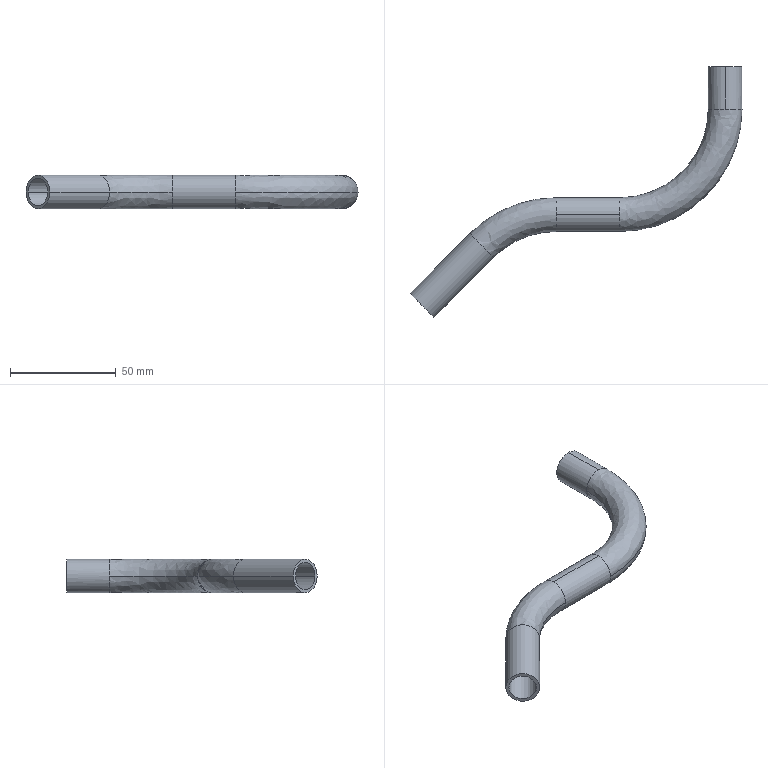Part | STEP file | copper tube 10_default_machined_ | 1 solid | 22 faces | box 157.296 x 118.586 x 16 mm | volume 14200 mm3 | cylinder 12 | spline 8 | plane 2 | commonest cylinder face diameters 13 x6 16 x6